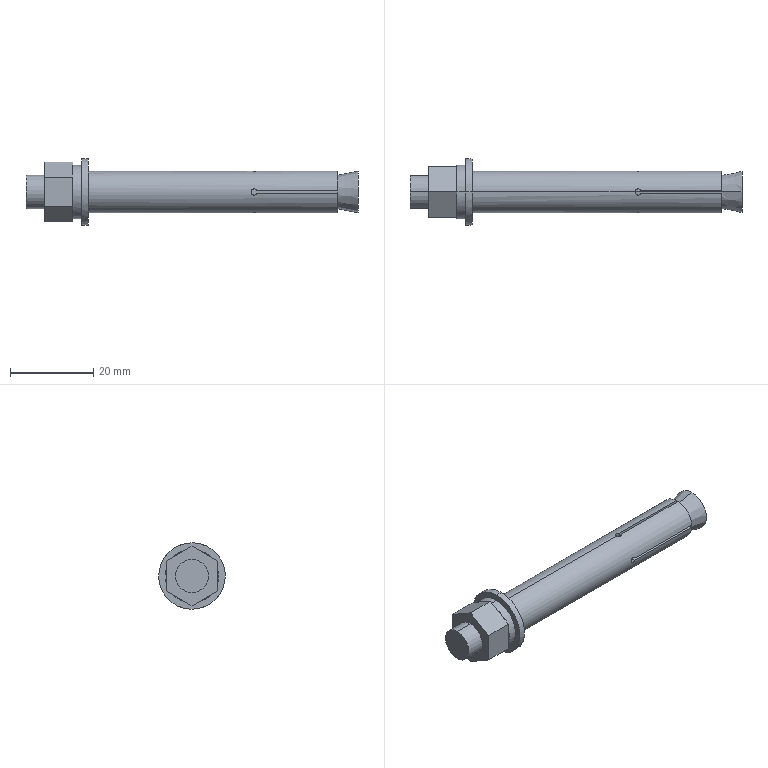Part | STEP file | 103000016257 | 3 solids | 59 faces | box 80 x 16 x 16 mm | volume 6519 mm3 | plane 29 | cylinder 28 | cone 2 | commonest cylinder face diameters 1.5 x10 8 x4 8.68 x3 12.88 x3 8.2 x2 9 x2